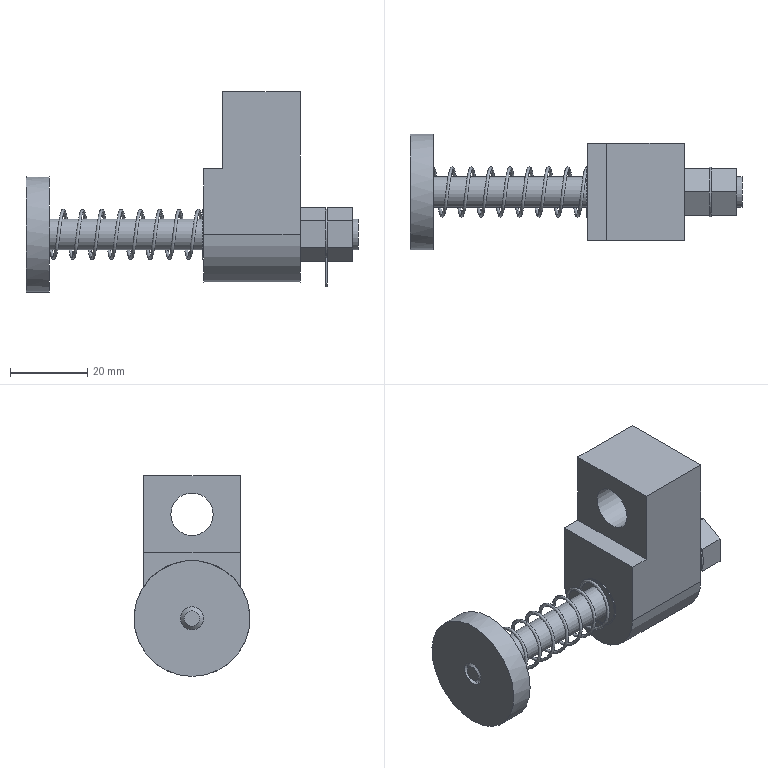Part | NX | features 1605242043 2 | 1 solid | 77 faces | box 86 x 30 x 52 mm | volume 33018 mm3 | plane 60 | cylinder 15 | spline 1 | cone 1 | commonest cylinder face diameters 8 x3 13 x3 12.25 x2 2.5 x1 6 x1 8.1 x1